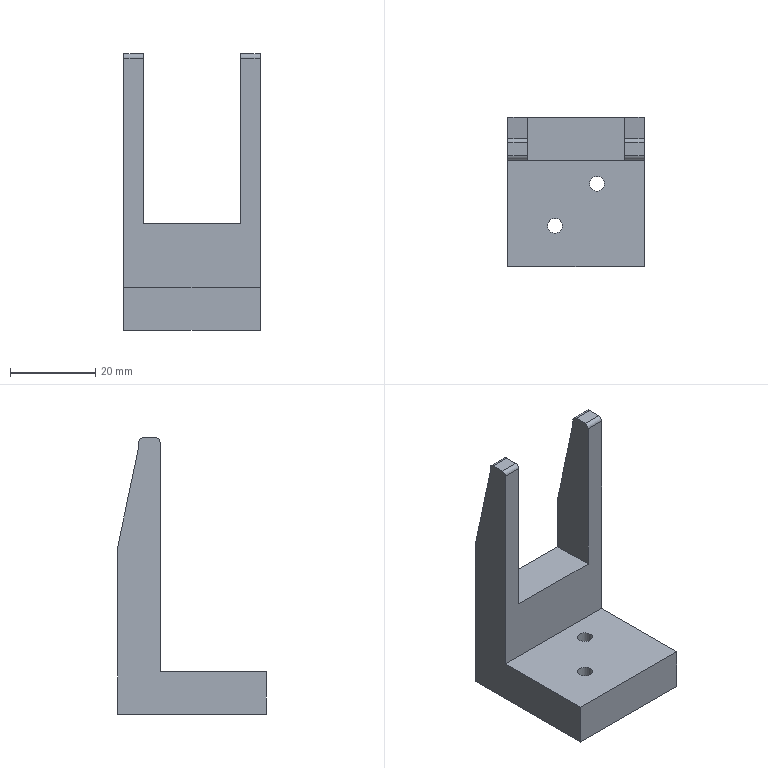Part | NX | features BREP 1 | 1 solid | 26 faces | box 32 x 35 x 65 mm | volume 18690 mm3 | plane 16 | cylinder 8 | cone 2 | commonest cylinder face diameters 2 x4 3 x2 3.5 x2
STEP:
#1=CARTESIAN_POINT('',(-16.,10.,65.));
#2=VERTEX_POINT('',#1);
#3=CARTESIAN_POINT('',(-16.,7.,65.));
#4=VERTEX_POINT('',#3);
#5=CARTESIAN_POINT('',(-16.,-19.,65.));
#6=DIRECTION('',(0.,-1.,0.));
#7=VECTOR('',#6,1000.);
#8=LINE('',#5,#7);
#9=EDGE_CURVE('',#2,#4,#8,.T.);
#10=ORIENTED_EDGE('',*,*,#9,.T.);
#11=CARTESIAN_POINT('',(-11.5,7.,65.));
#12=VERTEX_POINT('',#11);
#13=CARTESIAN_POINT('',(-11.5,7.,65.));
#14=DIRECTION('',(1.,0.,0.));
#15=VECTOR('',#14,1000.);
#16=LINE('',#13,#15);
#17=EDGE_CURVE('',#4,#12,#16,.T.);
#18=ORIENTED_EDGE('',*,*,#17,.T.);
#19=CARTESIAN_POINT('',(-11.5,10.,65.));
#20=VERTEX_POINT('',#19);
#21=CARTESIAN_POINT('',(-11.5,16.,65.));
#22=DIRECTION('',(0.,-1.,0.));
#23=VECTOR('',#22,1000.);
#24=LINE('',#21,#23);
#25=EDGE_CURVE('',#20,#12,#24,.T.);
#26=ORIENTED_EDGE('',*,*,#25,.F.);
#27=CARTESIAN_POINT('',(0.,10.,65.));
#28=DIRECTION('',(-1.,0.,0.));
#29=VECTOR('',#28,1000.);
#30=LINE('',#27,#29);
#31=EDGE_CURVE('',#20,#2,#30,.T.);
#32=ORIENTED_EDGE('',*,*,#31,.T.);
#33=EDGE_LOOP('',(#10,#18,#26,#32));
#34=FACE_BOUND('',#33,.T.);
#35=CARTESIAN_POINT('',(0.,0.,65.));
#36=DIRECTION('',(0.,0.,-1.));
#37=DIRECTION('',(1.,0.,0.));
#38=AXIS2_PLACEMENT_3D('',#35,#36,#37);
#39=PLANE('',#38);
#40=ADVANCED_FACE('',(#34),#39,.F.);
#41=CARTESIAN_POINT('',(-16.,11.,63.));
#42=VERTEX_POINT('',#41);
#43=CARTESIAN_POINT('',(-11.5,11.,63.));
#44=VERTEX_POINT('',#43);
#45=CARTESIAN_POINT('',(-81.49,11.,63.));
#46=DIRECTION('',(1.,0.,0.));
#47=VECTOR('',#46,1000.);
#48=LINE('',#45,#47);
#49=EDGE_CURVE('',#42,#44,#48,.T.);
#50=ORIENTED_EDGE('',*,*,#49,.T.);
#51=CARTESIAN_POINT('',(-11.5,16.,39.25));
#52=VERTEX_POINT('',#51);
#53=CARTESIAN_POINT('',(-11.5,23.233,4.891));
#54=DIRECTION('',(0.,0.206,-0.9785));
#55=VECTOR('',#54,1000.);
#56=LINE('',#53,#55);
#57=EDGE_CURVE('',#44,#52,#56,.T.);
#58=ORIENTED_EDGE('',*,*,#57,.T.);
#59=CARTESIAN_POINT('',(-16.,16.,39.25));
#60=VERTEX_POINT('',#59);
#61=CARTESIAN_POINT('',(-81.49,16.,39.25));
#62=DIRECTION('',(1.,0.,0.));
#63=VECTOR('',#62,1000.);
#64=LINE('',#61,#63);
#65=EDGE_CURVE('',#60,#52,#64,.T.);
#66=ORIENTED_EDGE('',*,*,#65,.F.);
#67=CARTESIAN_POINT('',(-16.,23.233,4.891));
#68=DIRECTION('',(0.,-0.206,0.9785));
#69=VECTOR('',#68,1000.);
#70=LINE('',#67,#69);
#71=EDGE_CURVE('',#60,#42,#70,.T.);
#72=ORIENTED_EDGE('',*,*,#71,.T.);
#73=EDGE_LOOP('',(#50,#58,#66,#72));
#74=FACE_BOUND('',#73,.T.);
#75=CARTESIAN_POINT('',(-81.49,23.233,4.891));
#76=DIRECTION('',(0.,-0.9785,-0.206));
#77=DIRECTION('',(0.,-0.206,0.9785));
#78=AXIS2_PLACEMENT_3D('',#75,#76,#77);
#79=PLANE('',#78);
#80=ADVANCED_FACE('',(#74),#79,.F.);
#81=CARTESIAN_POINT('',(-16.,11.,64.));
#82=VERTEX_POINT('',#81);
#83=CARTESIAN_POINT('',(-16.,11.,0.));
#84=DIRECTION('',(0.,0.,1.));
#85=VECTOR('',#84,1000.);
#86=LINE('',#83,#85);
#87=EDGE_CURVE('',#42,#82,#86,.T.);
#88=ORIENTED_EDGE('',*,*,#87,.T.);
#89=CARTESIAN_POINT('',(-11.5,11.,64.));
#90=VERTEX_POINT('',#89);
#91=CARTESIAN_POINT('',(-81.49,11.,64.));
#92=DIRECTION('',(1.,0.,0.));
#93=VECTOR('',#92,1000.);
#94=LINE('',#91,#93);
#95=EDGE_CURVE('',#82,#90,#94,.T.);
#96=ORIENTED_EDGE('',*,*,#95,.T.);
#97=CARTESIAN_POINT('',(-11.5,11.,0.));
#98=DIRECTION('',(0.,0.,-1.));
#99=VECTOR('',#98,1000.);
#100=LINE('',#97,#99);
#101=EDGE_CURVE('',#90,#44,#100,.T.);
#102=ORIENTED_EDGE('',*,*,#101,.T.);
#103=ORIENTED_EDGE('',*,*,#49,.F.);
#104=EDGE_LOOP('',(#88,#96,#102,#103));
#105=FACE_BOUND('',#104,.T.);
#106=CARTESIAN_POINT('',(-81.49,11.,0.));
#107=DIRECTION('',(0.,-1.,0.));
#108=DIRECTION('',(0.,0.,1.));
#109=AXIS2_PLACEMENT_3D('',#106,#107,#108);
#110=PLANE('',#109);
#111=ADVANCED_FACE('',(#105),#110,.F.);
#112=CARTESIAN_POINT('',(16.,7.,65.));
#113=VERTEX_POINT('',#112);
#114=CARTESIAN_POINT('',(16.,10.,65.));
#115=VERTEX_POINT('',#114);
#116=CARTESIAN_POINT('',(16.,-19.,65.));
#117=DIRECTION('',(0.,1.,0.));
#118=VECTOR('',#117,1000.);
#119=LINE('',#116,#118);
#120=EDGE_CURVE('',#113,#115,#119,.T.);
#121=ORIENTED_EDGE('',*,*,#120,.F.);
#122=CARTESIAN_POINT('',(16.,6.,64.));
#123=VERTEX_POINT('',#122);
#124=CARTESIAN_POINT('',(16.,7.,64.));
#125=DIRECTION('',(1.,0.,0.));
#126=DIRECTION('',(0.,0.,1.));
#127=AXIS2_PLACEMENT_3D('',#124,#125,#126);
#128=CIRCLE('',#127,1.);
#129=EDGE_CURVE('',#113,#123,#128,.T.);
#130=ORIENTED_EDGE('',*,*,#129,.T.);
#131=CARTESIAN_POINT('',(16.,6.,10.));
#132=VERTEX_POINT('',#131);
#133=CARTESIAN_POINT('',(16.,6.,0.));
#134=DIRECTION('',(0.,0.,-1.));
#135=VECTOR('',#134,1000.);
#136=LINE('',#133,#135);
#137=EDGE_CURVE('',#123,#132,#136,.T.);
#138=ORIENTED_EDGE('',*,*,#137,.T.);
#139=CARTESIAN_POINT('',(16.,-19.,10.));
#140=VERTEX_POINT('',#139);
#141=CARTESIAN_POINT('',(16.,0.,10.));
#142=DIRECTION('',(0.,1.,0.));
#143=VECTOR('',#142,1000.);
#144=LINE('',#141,#143);
#145=EDGE_CURVE('',#140,#132,#144,.T.);
#146=ORIENTED_EDGE('',*,*,#145,.F.);
#147=CARTESIAN_POINT('',(16.,-19.,0.));
#148=VERTEX_POINT('',#147);
#149=CARTESIAN_POINT('',(16.,-19.,65.));
#150=DIRECTION('',(0.,0.,-1.));
#151=VECTOR('',#150,1000.);
#152=LINE('',#149,#151);
#153=EDGE_CURVE('',#140,#148,#152,.T.);
#154=ORIENTED_EDGE('',*,*,#153,.T.);
#155=CARTESIAN_POINT('',(16.,16.,0.));
#156=VERTEX_POINT('',#155);
#157=CARTESIAN_POINT('',(16.,-19.,0.));
#158=DIRECTION('',(0.,1.,0.));
#159=VECTOR('',#158,1000.);
#160=LINE('',#157,#159);
#161=EDGE_CURVE('',#148,#156,#160,.T.);
#162=ORIENTED_EDGE('',*,*,#161,.T.);
#163=CARTESIAN_POINT('',(16.,16.,39.25));
#164=VERTEX_POINT('',#163);
#165=CARTESIAN_POINT('',(16.,16.,0.));
#166=DIRECTION('',(0.,0.,-1.));
#167=VECTOR('',#166,1000.);
#168=LINE('',#165,#167);
#169=EDGE_CURVE('',#164,#156,#168,.T.);
#170=ORIENTED_EDGE('',*,*,#169,.F.);
#171=CARTESIAN_POINT('',(16.,11.,63.));
#172=VERTEX_POINT('',#171);
#173=CARTESIAN_POINT('',(16.,23.233,4.891));
#174=DIRECTION('',(0.,0.206,-0.9785));
#175=VECTOR('',#174,1000.);
#176=LINE('',#173,#175);
#177=EDGE_CURVE('',#172,#164,#176,.T.);
#178=ORIENTED_EDGE('',*,*,#177,.F.);
#179=CARTESIAN_POINT('',(16.,11.,64.));
#180=VERTEX_POINT('',#179);
#181=CARTESIAN_POINT('',(16.,11.,0.));
#182=DIRECTION('',(0.,0.,-1.));
#183=VECTOR('',#182,1000.);
#184=LINE('',#181,#183);
#185=EDGE_CURVE('',#180,#172,#184,.T.);
#186=ORIENTED_EDGE('',*,*,#185,.F.);
#187=CARTESIAN_POINT('',(16.,10.,64.));
#188=DIRECTION('',(1.,0.,0.));
#189=DIRECTION('',(0.,0.,1.));
#190=AXIS2_PLACEMENT_3D('',#187,#188,#189);
#191=CIRCLE('',#190,1.);
#192=EDGE_CURVE('',#180,#115,#191,.T.);
#193=ORIENTED_EDGE('',*,*,#192,.T.);
#194=EDGE_LOOP('',(#121,#130,#138,#146,#154,#162,#170,#178,#186,#193));
#195=FACE_BOUND('',#194,.T.);
#196=CARTESIAN_POINT('',(16.,-19.,65.));
#197=DIRECTION('',(-1.,0.,0.));
#198=DIRECTION('',(0.,0.,-1.));
#199=AXIS2_PLACEMENT_3D('',#196,#197,#198);
#200=PLANE('',#199);
#201=ADVANCED_FACE('',(#195),#200,.F.);
#202=CARTESIAN_POINT('',(-16.,6.,10.));
#203=VERTEX_POINT('',#202);
#204=CARTESIAN_POINT('',(-16.,6.,64.));
#205=VERTEX_POINT('',#204);
#206=CARTESIAN_POINT('',(-16.,6.,0.));
#207=DIRECTION('',(0.,0.,1.));
#208=VECTOR('',#207,1000.);
#209=LINE('',#206,#208);
#210=EDGE_CURVE('',#203,#205,#209,.T.);
#211=ORIENTED_EDGE('',*,*,#210,.T.);
#212=CARTESIAN_POINT('',(-16.,7.,64.));
#213=DIRECTION('',(-1.,0.,0.));
#214=DIRECTION('',(0.,0.,-1.));
#215=AXIS2_PLACEMENT_3D('',#212,#213,#214);
#216=CIRCLE('',#215,1.);
#217=EDGE_CURVE('',#205,#4,#216,.T.);
#218=ORIENTED_EDGE('',*,*,#217,.T.);
#219=ORIENTED_EDGE('',*,*,#9,.F.);
#220=CARTESIAN_POINT('',(-16.,10.,64.));
#221=DIRECTION('',(-1.,0.,0.));
#222=DIRECTION('',(0.,0.,-1.));
#223=AXIS2_PLACEMENT_3D('',#220,#221,#222);
#224=CIRCLE('',#223,1.);
#225=EDGE_CURVE('',#2,#82,#224,.T.);
#226=ORIENTED_EDGE('',*,*,#225,.T.);
#227=ORIENTED_EDGE('',*,*,#87,.F.);
#228=ORIENTED_EDGE('',*,*,#71,.F.);
#229=CARTESIAN_POINT('',(-16.,16.,0.));
#230=VERTEX_POINT('',#229);
#231=CARTESIAN_POINT('',(-16.,16.,0.));
#232=DIRECTION('',(0.,0.,1.));
#233=VECTOR('',#232,1000.);
#234=LINE('',#231,#233);
#235=EDGE_CURVE('',#230,#60,#234,.T.);
#236=ORIENTED_EDGE('',*,*,#235,.F.);
#237=CARTESIAN_POINT('',(-16.,-19.,0.));
#238=VERTEX_POINT('',#237);
#239=CARTESIAN_POINT('',(-16.,-19.,0.));
#240=DIRECTION('',(0.,-1.,0.));
#241=VECTOR('',#240,1000.);
#242=LINE('',#239,#241);
#243=EDGE_CURVE('',#230,#238,#242,.T.);
#244=ORIENTED_EDGE('',*,*,#243,.T.);
#245=CARTESIAN_POINT('',(-16.,-19.,10.));
#246=VERTEX_POINT('',#245);
#247=CARTESIAN_POINT('',(-16.,-19.,65.));
#248=DIRECTION('',(0.,0.,-1.));
#249=VECTOR('',#248,1000.);
#250=LINE('',#247,#249);
#251=EDGE_CURVE('',#246,#238,#250,.T.);
#252=ORIENTED_EDGE('',*,*,#251,.F.);
#253=CARTESIAN_POINT('',(-16.,0.,10.));
#254=DIRECTION('',(0.,-1.,0.));
#255=VECTOR('',#254,1000.);
#256=LINE('',#253,#255);
#257=EDGE_CURVE('',#203,#246,#256,.T.);
#258=ORIENTED_EDGE('',*,*,#257,.F.);
#259=EDGE_LOOP('',(#211,#218,#219,#226,#227,#228,#236,#244,#252,#258));
#260=FACE_BOUND('',#259,.T.);
#261=CARTESIAN_POINT('',(-16.,-19.,65.));
#262=DIRECTION('',(1.,0.,0.));
#263=DIRECTION('',(0.,0.,1.));
#264=AXIS2_PLACEMENT_3D('',#261,#262,#263);
#265=PLANE('',#264);
#266=ADVANCED_FACE('',(#260),#265,.F.);
#267=CARTESIAN_POINT('',(11.5,10.,65.));
#268=VERTEX_POINT('',#267);
#269=CARTESIAN_POINT('',(11.5,7.,65.));
#270=VERTEX_POINT('',#269);
#271=CARTESIAN_POINT('',(11.5,16.,65.));
#272=DIRECTION('',(0.,-1.,0.));
#273=VECTOR('',#272,1000.);
#274=LINE('',#271,#273);
#275=EDGE_CURVE('',#268,#270,#274,.T.);
#276=ORIENTED_EDGE('',*,*,#275,.T.);
#277=CARTESIAN_POINT('',(16.,7.,65.));
#278=DIRECTION('',(1.,0.,0.));
#279=VECTOR('',#278,1000.);
#280=LINE('',#277,#279);
#281=EDGE_CURVE('',#270,#113,#280,.T.);
#282=ORIENTED_EDGE('',*,*,#281,.T.);
#283=ORIENTED_EDGE('',*,*,#120,.T.);
#284=CARTESIAN_POINT('',(0.,10.,65.));
#285=DIRECTION('',(-1.,0.,0.));
#286=VECTOR('',#285,1000.);
#287=LINE('',#284,#286);
#288=EDGE_CURVE('',#115,#268,#287,.T.);
#289=ORIENTED_EDGE('',*,*,#288,.T.);
#290=EDGE_LOOP('',(#276,#282,#283,#289));
#291=FACE_BOUND('',#290,.T.);
#292=CARTESIAN_POINT('',(0.,0.,65.));
#293=DIRECTION('',(0.,0.,-1.));
#294=DIRECTION('',(1.,0.,0.));
#295=AXIS2_PLACEMENT_3D('',#292,#293,#294);
#296=PLANE('',#295);
#297=ADVANCED_FACE('',(#291),#296,.F.);
#298=ORIENTED_EDGE('',*,*,#153,.F.);
#299=CARTESIAN_POINT('',(-81.49,-19.,10.));
#300=DIRECTION('',(1.,0.,0.));
#301=VECTOR('',#300,1000.);
#302=LINE('',#299,#301);
#303=EDGE_CURVE('',#246,#140,#302,.T.);
#304=ORIENTED_EDGE('',*,*,#303,.F.);
#305=ORIENTED_EDGE('',*,*,#251,.T.);
#306=CARTESIAN_POINT('',(-16.,-19.,0.));
#307=DIRECTION('',(1.,0.,0.));
#308=VECTOR('',#307,1000.);
#309=LINE('',#306,#308);
#310=EDGE_CURVE('',#238,#148,#309,.T.);
#311=ORIENTED_EDGE('',*,*,#310,.T.);
#312=EDGE_LOOP('',(#298,#304,#305,#311));
#313=FACE_BOUND('',#312,.T.);
#314=CARTESIAN_POINT('',(-16.,-19.,65.));
#315=DIRECTION('',(0.,1.,0.));
#316=DIRECTION('',(0.,0.,-1.));
#317=AXIS2_PLACEMENT_3D('',#314,#315,#316);
#318=PLANE('',#317);
#319=ADVANCED_FACE('',(#313),#318,.F.);
#320=CARTESIAN_POINT('',(3.2,0.4497,0.));
#321=VERTEX_POINT('',#320);
#322=CARTESIAN_POINT('',(4.95,0.4497,0.));
#323=DIRECTION('',(0.,0.,-1.));
#324=DIRECTION('',(-1.,0.,0.));
#325=AXIS2_PLACEMENT_3D('',#322,#323,#324);
#326=CIRCLE('',#325,1.75);
#327=EDGE_CURVE('',#321,#321,#326,.T.);
#328=ORIENTED_EDGE('',*,*,#327,.F.);
#329=EDGE_LOOP('',(#328));
#330=FACE_BOUND('',#329,.T.);
#331=CARTESIAN_POINT('',(-6.7,-9.45,0.));
#332=VERTEX_POINT('',#331);
#333=CARTESIAN_POINT('',(-4.95,-9.45,0.));
#334=DIRECTION('',(0.,0.,-1.));
#335=DIRECTION('',(-1.,0.,0.));
#336=AXIS2_PLACEMENT_3D('',#333,#334,#335);
#337=CIRCLE('',#336,1.75);
#338=EDGE_CURVE('',#332,#332,#337,.T.);
#339=ORIENTED_EDGE('',*,*,#338,.F.);
#340=EDGE_LOOP('',(#339));
#341=FACE_BOUND('',#340,.T.);
#342=CARTESIAN_POINT('',(3.45,-9.45,0.));
#343=VERTEX_POINT('',#342);
#344=CARTESIAN_POINT('',(4.95,-9.45,0.));
#345=DIRECTION('',(0.,0.,-1.));
#346=DIRECTION('',(-1.,0.,0.));
#347=AXIS2_PLACEMENT_3D('',#344,#345,#346);
#348=CIRCLE('',#347,1.5);
#349=EDGE_CURVE('',#343,#343,#348,.T.);
#350=ORIENTED_EDGE('',*,*,#349,.F.);
#351=EDGE_LOOP('',(#350));
#352=FACE_BOUND('',#351,.T.);
#353=CARTESIAN_POINT('',(-6.45,0.4497,0.));
#354=VERTEX_POINT('',#353);
#355=CARTESIAN_POINT('',(-4.95,0.4497,0.));
#356=DIRECTION('',(0.,0.,-1.));
#357=DIRECTION('',(-1.,0.,0.));
#358=AXIS2_PLACEMENT_3D('',#355,#356,#357);
#359=CIRCLE('',#358,1.5);
#360=EDGE_CURVE('',#354,#354,#359,.T.);
#361=ORIENTED_EDGE('',*,*,#360,.F.);
#362=EDGE_LOOP('',(#361));
#363=FACE_BOUND('',#362,.T.);
#364=CARTESIAN_POINT('',(-81.49,16.,0.));
#365=DIRECTION('',(1.,0.,0.));
#366=VECTOR('',#365,1000.);
#367=LINE('',#364,#366);
#368=EDGE_CURVE('',#230,#156,#367,.T.);
#369=ORIENTED_EDGE('',*,*,#368,.T.);
#370=ORIENTED_EDGE('',*,*,#161,.F.);
#371=ORIENTED_EDGE('',*,*,#310,.F.);
#372=ORIENTED_EDGE('',*,*,#243,.F.);
#373=EDGE_LOOP('',(#369,#370,#371,#372));
#374=FACE_BOUND('',#373,.T.);
#375=CARTESIAN_POINT('',(0.,0.,0.));
#376=DIRECTION('',(0.,0.,-1.));
#377=DIRECTION('',(1.,0.,0.));
#378=AXIS2_PLACEMENT_3D('',#375,#376,#377);
#379=PLANE('',#378);
#380=ADVANCED_FACE('',(#330,#341,#352,#363,#374),#379,.T.);
#381=ORIENTED_EDGE('',*,*,#65,.T.);
#382=CARTESIAN_POINT('',(-11.5,16.,25.));
#383=VERTEX_POINT('',#382);
#384=CARTESIAN_POINT('',(-11.5,16.,65.));
#385=DIRECTION('',(0.,0.,-1.));
#386=VECTOR('',#385,1000.);
#387=LINE('',#384,#386);
#388=EDGE_CURVE('',#52,#383,#387,.T.);
#389=ORIENTED_EDGE('',*,*,#388,.T.);
#390=CARTESIAN_POINT('',(11.5,16.,25.));
#391=VERTEX_POINT('',#390);
#392=CARTESIAN_POINT('',(-11.5,16.,25.));
#393=DIRECTION('',(1.,0.,0.));
#394=VECTOR('',#393,1000.);
#395=LINE('',#392,#394);
#396=EDGE_CURVE('',#383,#391,#395,.T.);
#397=ORIENTED_EDGE('',*,*,#396,.T.);
#398=CARTESIAN_POINT('',(11.5,16.,39.25));
#399=VERTEX_POINT('',#398);
#400=CARTESIAN_POINT('',(11.5,16.,65.));
#401=DIRECTION('',(0.,0.,1.));
#402=VECTOR('',#401,1000.);
#403=LINE('',#400,#402);
#404=EDGE_CURVE('',#391,#399,#403,.T.);
#405=ORIENTED_EDGE('',*,*,#404,.T.);
#406=CARTESIAN_POINT('',(-81.49,16.,39.25));
#407=DIRECTION('',(1.,0.,0.));
#408=VECTOR('',#407,1000.);
#409=LINE('',#406,#408);
#410=EDGE_CURVE('',#399,#164,#409,.T.);
#411=ORIENTED_EDGE('',*,*,#410,.T.);
#412=ORIENTED_EDGE('',*,*,#169,.T.);
#413=ORIENTED_EDGE('',*,*,#368,.F.);
#414=ORIENTED_EDGE('',*,*,#235,.T.);
#415=EDGE_LOOP('',(#381,#389,#397,#405,#411,#412,#413,#414));
#416=FACE_BOUND('',#415,.T.);
#417=CARTESIAN_POINT('',(-81.49,16.,0.));
#418=DIRECTION('',(0.,-1.,0.));
#419=DIRECTION('',(0.,0.,1.));
#420=AXIS2_PLACEMENT_3D('',#417,#418,#419);
#421=PLANE('',#420);
#422=ADVANCED_FACE('',(#416),#421,.F.);
#423=ORIENTED_EDGE('',*,*,#410,.F.);
#424=CARTESIAN_POINT('',(11.5,11.,63.));
#425=VERTEX_POINT('',#424);
#426=CARTESIAN_POINT('',(11.5,23.233,4.891));
#427=DIRECTION('',(0.,-0.206,0.9785));
#428=VECTOR('',#427,1000.);
#429=LINE('',#426,#428);
#430=EDGE_CURVE('',#399,#425,#429,.T.);
#431=ORIENTED_EDGE('',*,*,#430,.T.);
#432=CARTESIAN_POINT('',(-81.49,11.,63.));
#433=DIRECTION('',(1.,0.,0.));
#434=VECTOR('',#433,1000.);
#435=LINE('',#432,#434);
#436=EDGE_CURVE('',#425,#172,#435,.T.);
#437=ORIENTED_EDGE('',*,*,#436,.T.);
#438=ORIENTED_EDGE('',*,*,#177,.T.);
#439=EDGE_LOOP('',(#423,#431,#437,#438));
#440=FACE_BOUND('',#439,.T.);
#441=CARTESIAN_POINT('',(-81.49,23.233,4.891));
#442=DIRECTION('',(0.,-0.9785,-0.206));
#443=DIRECTION('',(0.,-0.206,0.9785));
#444=AXIS2_PLACEMENT_3D('',#441,#442,#443);
#445=PLANE('',#444);
#446=ADVANCED_FACE('',(#440),#445,.F.);
#447=CARTESIAN_POINT('',(11.5,11.,64.));
#448=VERTEX_POINT('',#447);
#449=CARTESIAN_POINT('',(11.5,11.,0.));
#450=DIRECTION('',(0.,0.,1.));
#451=VECTOR('',#450,1000.);
#452=LINE('',#449,#451);
#453=EDGE_CURVE('',#425,#448,#452,.T.);
#454=ORIENTED_EDGE('',*,*,#453,.T.);
#455=CARTESIAN_POINT('',(-81.49,11.,64.));
#456=DIRECTION('',(1.,0.,0.));
#457=VECTOR('',#456,1000.);
#458=LINE('',#455,#457);
#459=EDGE_CURVE('',#448,#180,#458,.T.);
#460=ORIENTED_EDGE('',*,*,#459,.T.);
#461=ORIENTED_EDGE('',*,*,#185,.T.);
#462=ORIENTED_EDGE('',*,*,#436,.F.);
#463=EDGE_LOOP('',(#454,#460,#461,#462));
#464=FACE_BOUND('',#463,.T.);
#465=CARTESIAN_POINT('',(-81.49,11.,0.));
#466=DIRECTION('',(0.,-1.,0.));
#467=DIRECTION('',(0.,0.,1.));
#468=AXIS2_PLACEMENT_3D('',#465,#466,#467);
#469=PLANE('',#468);
#470=ADVANCED_FACE('',(#464),#469,.F.);
#471=CARTESIAN_POINT('',(-11.5,6.,64.));
#472=VERTEX_POINT('',#471);
#473=CARTESIAN_POINT('',(-11.5,6.,25.));
#474=VERTEX_POINT('',#473);
#475=CARTESIAN_POINT('',(-11.5,6.,65.));
#476=DIRECTION('',(0.,0.,-1.));
#477=VECTOR('',#476,1000.);
#478=LINE('',#475,#477);
#479=EDGE_CURVE('',#472,#474,#478,.T.);
#480=ORIENTED_EDGE('',*,*,#479,.F.);
#481=CARTESIAN_POINT('',(-16.,6.,64.));
#482=DIRECTION('',(-1.,0.,0.));
#483=VECTOR('',#482,1000.);
#484=LINE('',#481,#483);
#485=EDGE_CURVE('',#472,#205,#484,.T.);
#486=ORIENTED_EDGE('',*,*,#485,.T.);
#487=ORIENTED_EDGE('',*,*,#210,.F.);
#488=CARTESIAN_POINT('',(-81.49,6.,10.));
#489=DIRECTION('',(1.,0.,0.));
#490=VECTOR('',#489,1000.);
#491=LINE('',#488,#490);
#492=EDGE_CURVE('',#203,#132,#491,.T.);
#493=ORIENTED_EDGE('',*,*,#492,.T.);
#494=ORIENTED_EDGE('',*,*,#137,.F.);
#495=CARTESIAN_POINT('',(11.5,6.,64.));
#496=VERTEX_POINT('',#495);
#497=CARTESIAN_POINT('',(11.5,6.,64.));
#498=DIRECTION('',(-1.,0.,0.));
#499=VECTOR('',#498,1000.);
#500=LINE('',#497,#499);
#501=EDGE_CURVE('',#123,#496,#500,.T.);
#502=ORIENTED_EDGE('',*,*,#501,.T.);
#503=CARTESIAN_POINT('',(11.5,6.,25.));
#504=VERTEX_POINT('',#503);
#505=CARTESIAN_POINT('',(11.5,6.,65.));
#506=DIRECTION('',(0.,0.,1.));
#507=VECTOR('',#506,1000.);
#508=LINE('',#505,#507);
#509=EDGE_CURVE('',#504,#496,#508,.T.);
#510=ORIENTED_EDGE('',*,*,#509,.F.);
#511=CARTESIAN_POINT('',(-11.5,6.,25.));
#512=DIRECTION('',(1.,0.,0.));
#513=VECTOR('',#512,1000.);
#514=LINE('',#511,#513);
#515=EDGE_CURVE('',#474,#504,#514,.T.);
#516=ORIENTED_EDGE('',*,*,#515,.F.);
#517=EDGE_LOOP('',(#480,#486,#487,#493,#494,#502,#510,#516));
#518=FACE_BOUND('',#517,.T.);
#519=CARTESIAN_POINT('',(-81.49,6.,0.));
#520=DIRECTION('',(0.,-1.,0.));
#521=DIRECTION('',(0.,0.,1.));
#522=AXIS2_PLACEMENT_3D('',#519,#520,#521);
#523=PLANE('',#522);
#524=ADVANCED_FACE('',(#518),#523,.T.);
#525=CARTESIAN_POINT('',(3.2,0.4497,10.));
#526=VERTEX_POINT('',#525);
#527=CARTESIAN_POINT('',(4.95,0.4497,10.));
#528=DIRECTION('',(0.,0.,-1.));
#529=DIRECTION('',(-1.,0.,0.));
#530=AXIS2_PLACEMENT_3D('',#527,#528,#529);
#531=CIRCLE('',#530,1.75);
#532=EDGE_CURVE('',#526,#526,#531,.T.);
#533=ORIENTED_EDGE('',*,*,#532,.T.);
#534=EDGE_LOOP('',(#533));
#535=FACE_BOUND('',#534,.T.);
#536=CARTESIAN_POINT('',(-6.7,-9.45,10.));
#537=VERTEX_POINT('',#536);
#538=CARTESIAN_POINT('',(-4.95,-9.45,10.));
#539=DIRECTION('',(0.,0.,-1.));
#540=DIRECTION('',(-1.,0.,0.));
#541=AXIS2_PLACEMENT_3D('',#538,#539,#540);
#542=CIRCLE('',#541,1.75);
#543=EDGE_CURVE('',#537,#537,#542,.T.);
#544=ORIENTED_EDGE('',*,*,#543,.T.);
#545=EDGE_LOOP('',(#544));
#546=FACE_BOUND('',#545,.T.);
#547=ORIENTED_EDGE('',*,*,#257,.T.);
#548=ORIENTED_EDGE('',*,*,#303,.T.);
#549=ORIENTED_EDGE('',*,*,#145,.T.);
#550=ORIENTED_EDGE('',*,*,#492,.F.);
#551=EDGE_LOOP('',(#547,#548,#549,#550));
#552=FACE_BOUND('',#551,.T.);
#553=CARTESIAN_POINT('',(-81.49,0.,10.));
#554=DIRECTION('',(0.,0.,-1.));
#555=DIRECTION('',(1.,0.,0.));
#556=AXIS2_PLACEMENT_3D('',#553,#554,#555);
#557=PLANE('',#556);
#558=ADVANCED_FACE('',(#535,#546,#552),#557,.F.);
#559=ORIENTED_EDGE('',*,*,#25,.T.);
#560=CARTESIAN_POINT('',(-11.5,7.,64.));
#561=DIRECTION('',(1.,0.,0.));
#562=DIRECTION('',(0.,0.,1.));
#563=AXIS2_PLACEMENT_3D('',#560,#561,#562);
#564=CIRCLE('',#563,1.);
#565=EDGE_CURVE('',#12,#472,#564,.T.);
#566=ORIENTED_EDGE('',*,*,#565,.T.);
#567=ORIENTED_EDGE('',*,*,#479,.T.);
#568=CARTESIAN_POINT('',(-11.5,16.,25.));
#569=DIRECTION('',(0.,-1.,0.));
#570=VECTOR('',#569,1000.);
#571=LINE('',#568,#570);
#572=EDGE_CURVE('',#383,#474,#571,.T.);
#573=ORIENTED_EDGE('',*,*,#572,.F.);
#574=ORIENTED_EDGE('',*,*,#388,.F.);
#575=ORIENTED_EDGE('',*,*,#57,.F.);
#576=ORIENTED_EDGE('',*,*,#101,.F.);
#577=CARTESIAN_POINT('',(-11.5,10.,64.));
#578=DIRECTION('',(1.,0.,0.));
#579=DIRECTION('',(0.,0.,1.));
#580=AXIS2_PLACEMENT_3D('',#577,#578,#579);
#581=CIRCLE('',#580,1.);
#582=EDGE_CURVE('',#90,#20,#581,.T.);
#583=ORIENTED_EDGE('',*,*,#582,.T.);
#584=EDGE_LOOP('',(#559,#566,#567,#573,#574,#575,#576,#583));
#585=FACE_BOUND('',#584,.T.);
#586=CARTESIAN_POINT('',(-11.5,16.,65.));
#587=DIRECTION('',(-1.,0.,0.));
#588=DIRECTION('',(0.,0.,-1.));
#589=AXIS2_PLACEMENT_3D('',#586,#587,#588);
#590=PLANE('',#589);
#591=ADVANCED_FACE('',(#585),#590,.F.);
#592=ORIENTED_EDGE('',*,*,#509,.T.);
#593=CARTESIAN_POINT('',(11.5,7.,64.));
#594=DIRECTION('',(-1.,0.,0.));
#595=DIRECTION('',(0.,0.,-1.));
#596=AXIS2_PLACEMENT_3D('',#593,#594,#595);
#597=CIRCLE('',#596,1.);
#598=EDGE_CURVE('',#496,#270,#597,.T.);
#599=ORIENTED_EDGE('',*,*,#598,.T.);
#600=ORIENTED_EDGE('',*,*,#275,.F.);
#601=CARTESIAN_POINT('',(11.5,10.,64.));
#602=DIRECTION('',(-1.,0.,0.));
#603=DIRECTION('',(0.,0.,-1.));
#604=AXIS2_PLACEMENT_3D('',#601,#602,#603);
#605=CIRCLE('',#604,1.);
#606=EDGE_CURVE('',#268,#448,#605,.T.);
#607=ORIENTED_EDGE('',*,*,#606,.T.);
#608=ORIENTED_EDGE('',*,*,#453,.F.);
#609=ORIENTED_EDGE('',*,*,#430,.F.);
#610=ORIENTED_EDGE('',*,*,#404,.F.);
#611=CARTESIAN_POINT('',(11.5,16.,25.));
#612=DIRECTION('',(0.,-1.,0.));
#613=VECTOR('',#612,1000.);
#614=LINE('',#611,#613);
#615=EDGE_CURVE('',#391,#504,#614,.T.);
#616=ORIENTED_EDGE('',*,*,#615,.T.);
#617=EDGE_LOOP('',(#592,#599,#600,#607,#608,#609,#610,#616));
#618=FACE_BOUND('',#617,.T.);
#619=CARTESIAN_POINT('',(11.5,16.,65.));
#620=DIRECTION('',(1.,0.,0.));
#621=DIRECTION('',(0.,0.,1.));
#622=AXIS2_PLACEMENT_3D('',#619,#620,#621);
#623=PLANE('',#622);
#624=ADVANCED_FACE('',(#618),#623,.F.);
#625=ORIENTED_EDGE('',*,*,#515,.T.);
#626=ORIENTED_EDGE('',*,*,#615,.F.);
#627=ORIENTED_EDGE('',*,*,#396,.F.);
#628=ORIENTED_EDGE('',*,*,#572,.T.);
#629=EDGE_LOOP('',(#625,#626,#627,#628));
#630=FACE_BOUND('',#629,.T.);
#631=CARTESIAN_POINT('',(-11.5,16.,25.));
#632=DIRECTION('',(0.,0.,-1.));
#633=DIRECTION('',(1.,0.,0.));
#634=AXIS2_PLACEMENT_3D('',#631,#632,#633);
#635=PLANE('',#634);
#636=ADVANCED_FACE('',(#630),#635,.F.);
#637=CARTESIAN_POINT('',(-4.95,0.4497,6.901));
#638=VERTEX_POINT('',#637);
#639=VERTEX_LOOP('',#638);
#640=FACE_BOUND('',#639,.T.);
#641=CARTESIAN_POINT('',(-6.45,0.4497,6.));
#642=VERTEX_POINT('',#641);
#643=CARTESIAN_POINT('',(-4.95,0.4497,6.));
#644=DIRECTION('',(0.,0.,-1.));
#645=DIRECTION('',(-1.,0.,0.));
#646=AXIS2_PLACEMENT_3D('',#643,#644,#645);
#647=CIRCLE('',#646,1.5);
#648=EDGE_CURVE('',#642,#642,#647,.T.);
#649=ORIENTED_EDGE('',*,*,#648,.T.);
#650=EDGE_LOOP('',(#649));
#651=FACE_BOUND('',#650,.T.);
#652=CARTESIAN_POINT('',(-4.95,0.4497,6.));
#653=DIRECTION('',(0.,0.,-1.));
#654=DIRECTION('',(1.,0.,0.));
#655=AXIS2_PLACEMENT_3D('',#652,#653,#654);
#656=CONICAL_SURFACE('',#655,1.5,1.03);
#657=ADVANCED_FACE('',(#640,#651),#656,.F.);
#658=ORIENTED_EDGE('',*,*,#648,.F.);
#659=EDGE_LOOP('',(#658));
#660=FACE_BOUND('',#659,.T.);
#661=ORIENTED_EDGE('',*,*,#360,.T.);
#662=EDGE_LOOP('',(#661));
#663=FACE_BOUND('',#662,.T.);
#664=CARTESIAN_POINT('',(-4.95,0.4497,0.));
#665=DIRECTION('',(0.,0.,-1.));
#666=DIRECTION('',(1.,0.,0.));
#667=AXIS2_PLACEMENT_3D('',#664,#665,#666);
#668=CYLINDRICAL_SURFACE('',#667,1.5);
#669=ADVANCED_FACE('',(#660,#663),#668,.F.);
#670=CARTESIAN_POINT('',(4.95,-9.45,6.901));
#671=VERTEX_POINT('',#670);
#672=VERTEX_LOOP('',#671);
#673=FACE_BOUND('',#672,.T.);
#674=CARTESIAN_POINT('',(3.45,-9.45,6.));
#675=VERTEX_POINT('',#674);
#676=CARTESIAN_POINT('',(4.95,-9.45,6.));
#677=DIRECTION('',(0.,0.,-1.));
#678=DIRECTION('',(-1.,0.,0.));
#679=AXIS2_PLACEMENT_3D('',#676,#677,#678);
#680=CIRCLE('',#679,1.5);
#681=EDGE_CURVE('',#675,#675,#680,.T.);
#682=ORIENTED_EDGE('',*,*,#681,.T.);
#683=EDGE_LOOP('',(#682));
#684=FACE_BOUND('',#683,.T.);
#685=CARTESIAN_POINT('',(4.95,-9.45,6.));
#686=DIRECTION('',(0.,0.,-1.));
#687=DIRECTION('',(1.,0.,0.));
#688=AXIS2_PLACEMENT_3D('',#685,#686,#687);
#689=CONICAL_SURFACE('',#688,1.5,1.03);
#690=ADVANCED_FACE('',(#673,#684),#689,.F.);
#691=ORIENTED_EDGE('',*,*,#681,.F.);
#692=EDGE_LOOP('',(#691));
#693=FACE_BOUND('',#692,.T.);
#694=ORIENTED_EDGE('',*,*,#349,.T.);
#695=EDGE_LOOP('',(#694));
#696=FACE_BOUND('',#695,.T.);
#697=CARTESIAN_POINT('',(4.95,-9.45,0.));
#698=DIRECTION('',(0.,0.,-1.));
#699=DIRECTION('',(1.,0.,0.));
#700=AXIS2_PLACEMENT_3D('',#697,#698,#699);
#701=CYLINDRICAL_SURFACE('',#700,1.5);
#702=ADVANCED_FACE('',(#693,#696),#701,.F.);
#703=ORIENTED_EDGE('',*,*,#338,.T.);
#704=EDGE_LOOP('',(#703));
#705=FACE_BOUND('',#704,.T.);
#706=ORIENTED_EDGE('',*,*,#543,.F.);
#707=EDGE_LOOP('',(#706));
#708=FACE_BOUND('',#707,.T.);
#709=CARTESIAN_POINT('',(-4.95,-9.45,0.));
#710=DIRECTION('',(0.,0.,-1.));
#711=DIRECTION('',(1.,0.,0.));
#712=AXIS2_PLACEMENT_3D('',#709,#710,#711);
#713=CYLINDRICAL_SURFACE('',#712,1.75);
#714=ADVANCED_FACE('',(#705,#708),#713,.F.);
#715=ORIENTED_EDGE('',*,*,#327,.T.);
#716=EDGE_LOOP('',(#715));
#717=FACE_BOUND('',#716,.T.);
#718=ORIENTED_EDGE('',*,*,#532,.F.);
#719=EDGE_LOOP('',(#718));
#720=FACE_BOUND('',#719,.T.);
#721=CARTESIAN_POINT('',(4.95,0.4497,0.));
#722=DIRECTION('',(0.,0.,-1.));
#723=DIRECTION('',(1.,0.,0.));
#724=AXIS2_PLACEMENT_3D('',#721,#722,#723);
#725=CYLINDRICAL_SURFACE('',#724,1.75);
#726=ADVANCED_FACE('',(#717,#720),#725,.F.);
#727=ORIENTED_EDGE('',*,*,#217,.F.);
#728=ORIENTED_EDGE('',*,*,#485,.F.);
#729=ORIENTED_EDGE('',*,*,#565,.F.);
#730=ORIENTED_EDGE('',*,*,#17,.F.);
#731=EDGE_LOOP('',(#727,#728,#729,#730));
#732=FACE_BOUND('',#731,.T.);
#733=CARTESIAN_POINT('',(0.,7.,64.));
#734=DIRECTION('',(-1.,0.,0.));
#735=DIRECTION('',(0.,0.,-1.));
#736=AXIS2_PLACEMENT_3D('',#733,#734,#735);
#737=CYLINDRICAL_SURFACE('',#736,1.);
#738=ADVANCED_FACE('',(#732),#737,.T.);
#739=ORIENTED_EDGE('',*,*,#225,.F.);
#740=ORIENTED_EDGE('',*,*,#31,.F.);
#741=ORIENTED_EDGE('',*,*,#582,.F.);
#742=ORIENTED_EDGE('',*,*,#95,.F.);
#743=EDGE_LOOP('',(#739,#740,#741,#742));
#744=FACE_BOUND('',#743,.T.);
#745=CARTESIAN_POINT('',(-81.49,10.,64.));
#746=DIRECTION('',(1.,0.,0.));
#747=DIRECTION('',(0.,0.,1.));
#748=AXIS2_PLACEMENT_3D('',#745,#746,#747);
#749=CYLINDRICAL_SURFACE('',#748,1.);
#750=ADVANCED_FACE('',(#744),#749,.T.);
#751=ORIENTED_EDGE('',*,*,#598,.F.);
#752=ORIENTED_EDGE('',*,*,#501,.F.);
#753=ORIENTED_EDGE('',*,*,#129,.F.);
#754=ORIENTED_EDGE('',*,*,#281,.F.);
#755=EDGE_LOOP('',(#751,#752,#753,#754));
#756=FACE_BOUND('',#755,.T.);
#757=CARTESIAN_POINT('',(0.,7.,64.));
#758=DIRECTION('',(-1.,0.,0.));
#759=DIRECTION('',(0.,0.,-1.));
#760=AXIS2_PLACEMENT_3D('',#757,#758,#759);
#761=CYLINDRICAL_SURFACE('',#760,1.);
#762=ADVANCED_FACE('',(#756),#761,.T.);
#763=ORIENTED_EDGE('',*,*,#606,.F.);
#764=ORIENTED_EDGE('',*,*,#288,.F.);
#765=ORIENTED_EDGE('',*,*,#192,.F.);
#766=ORIENTED_EDGE('',*,*,#459,.F.);
#767=EDGE_LOOP('',(#763,#764,#765,#766));
#768=FACE_BOUND('',#767,.T.);
#769=CARTESIAN_POINT('',(-81.49,10.,64.));
#770=DIRECTION('',(1.,0.,0.));
#771=DIRECTION('',(0.,0.,1.));
#772=AXIS2_PLACEMENT_3D('',#769,#770,#771);
#773=CYLINDRICAL_SURFACE('',#772,1.);
#774=ADVANCED_FACE('',(#768),#773,.T.);
#775=CLOSED_SHELL('',(#40,#80,#111,#201,#266,#297,#319,#380,#422,#446,#470,#524,#558,#591,#624,#636,#657,#669,#690,#702,#714,#726,#738,#750,#762,#774));
#776=MANIFOLD_SOLID_BREP('',#775);
#777=(LENGTH_UNIT()NAMED_UNIT(*)SI_UNIT(.MILLI.,.METRE.));
#778=UNCERTAINTY_MEASURE_WITH_UNIT(LENGTH_MEASURE(0.00001),#777,'','');
#779=(NAMED_UNIT(*)PLANE_ANGLE_UNIT()SI_UNIT($,.RADIAN.));
#780=(NAMED_UNIT(*)SI_UNIT($,.STERADIAN.)SOLID_ANGLE_UNIT());
#781=(GEOMETRIC_REPRESENTATION_CONTEXT(3)GLOBAL_UNCERTAINTY_ASSIGNED_CONTEXT((#778))GLOBAL_UNIT_ASSIGNED_CONTEXT((#777,#779,#780))REPRESENTATION_CONTEXT('',''));
#782=ADVANCED_BREP_SHAPE_REPRESENTATION('',(#776),#781);